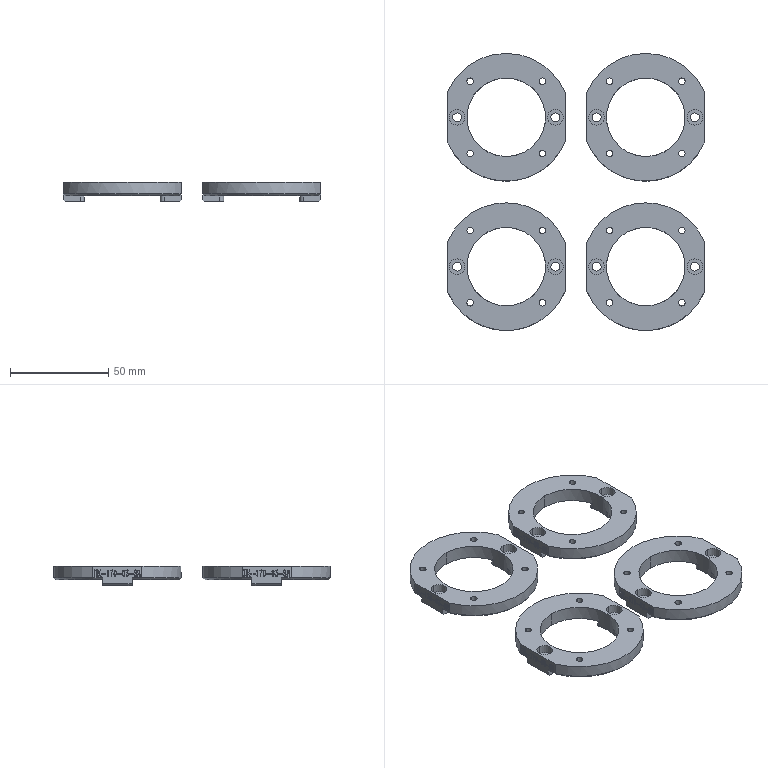NC program | NX | posted with a generic post | part box 131 x 141 x 10 mm
Lines 9684 to 11277 of 14293:
(FLOOR_WALL_COPY , TOOL : D10JING)
N19354 T14 M6
N19356 G54
N19358 G17 G0 G90 X-34.072 Y-75.973 S9500 M3
N19360 G43 Z30. H14
N19362 Z-2.
N19364 G94 G1 Z-3. F1000.
N19366 X-34.634 Y-75.
N19368 G3 X-35.5 Y-74.5 R1.
N19370 G2 X-69.103 Y-52.25 R36.5 F1500.
N19372 G1 X-69.5 Y-51.315
N19374 Y-51.
N19376 X-56.801
N19378 G3 X-49.31 Y-43.856 R7.5
N19380 X-21.69 Y-43.856 R15.
N19382 X-14.199 Y-51. R7.5
N19384 G1 X-1.5
N19386 Y-51.315
N19388 X-1.897 Y-52.25
N19390 G2 X-35.5 Y-74.5 R36.5
N19392 G1 Y-69.5
N19394 G2 X-61.351 Y-56. R31.5
N19396 G1 X-56.801
N19398 G3 X-48.703 Y-53.022 R12.5
N19400 X-22.297 Y-53.022 R20.
N19402 X-14.199 Y-56. R12.5
N19404 G1 X-9.649
N19406 G2 X-35.5 Y-69.5 R31.5
N19408 G1 Y-64.5
N19410 G2 X-50.519 Y-59.833 R26.5
N19412 G3 X-48.892 Y-59.111 R17.5
N19414 X-22.108 Y-59.111 R25.
N19416 X-20.481 Y-59.833 R17.5
N19418 G2 X-35.5 Y-64.5 R26.5
N19420 G3 X-36.366 Y-65. R1.
N19422 G1 Z-2.
N19424 G0 Z30.
N19426 X-48.796 Y-40.339
N19428 Z-2.
N19430 G1 Z-3. F1000.
N19432 X-49.643 Y-41.1
N19434 G3 X-49.953 Y-42.051 R1.
N19436 G2 X-56.801 Y-50.5 R7. F1500.
N19438 G1 X-69.5
N19440 G3 X-70.366 Y-51. R1.
N19442 G1 X-70.943 Y-52.
N19444 Z-2.
N19446 G0 Z30.
N19448 X-0.057
N19450 Z-2.
N19452 G1 Z-3. F1000.
N19454 X-0.634 Y-51.
N19456 G3 X-1.5 Y-50.5 R1.
N19458 G1 X-14.199 F1500.
N19460 G2 X-21.047 Y-42.051 R7.
N19462 G3 X-21.357 Y-41.1 R1.
N19464 G1 X-22.204 Y-40.339
N19466 Z-2.
N19468 G0 Z30.
N19470 X-36.928 Y-0.027
N19472 Z-2.
N19474 G1 Z-3. F1000.
N19476 X-36.366 Y-1.
N19478 G3 X-35.5 Y-1.5 R1.
N19480 G2 X-1.897 Y-23.75 R36.5 F1500.
N19482 G1 X-1.5 Y-24.685
N19484 Y-25.
N19486 X-14.199
N19488 G3 X-21.69 Y-32.144 R7.5
N19490 X-49.31 Y-32.144 R15.
N19492 X-56.801 Y-25. R7.5
N19494 G1 X-69.5
N19496 Y-24.685
N19498 X-69.103 Y-23.75
N19500 G2 X-35.5 Y-1.5 R36.5
N19502 G1 Y-6.5
N19504 G2 X-9.649 Y-20. R31.5
N19506 G1 X-14.199
N19508 G3 X-22.297 Y-22.978 R12.5
N19510 X-48.703 Y-22.978 R20.
N19512 X-56.801 Y-20. R12.5
N19514 G1 X-61.351
N19516 G2 X-35.5 Y-6.5 R31.5
N19518 G1 Y-11.5
N19520 G2 X-20.481 Y-16.167 R26.5
N19522 G3 X-22.108 Y-16.889 R17.5
N19524 X-48.892 Y-16.889 R25.
N19526 X-50.519 Y-16.167 R17.5
N19528 G2 X-35.5 Y-11.5 R26.5
N19530 G3 X-34.634 Y-11. R1.
N19532 G1 Z-2.
N19534 G0 Z30.
N19536 X-22.204 Y-35.661
N19538 Z-2.
N19540 G1 Z-3. F1000.
N19542 X-21.357 Y-34.9
N19544 G3 X-21.047 Y-33.949 R1.
N19546 G2 X-14.199 Y-25.5 R7. F1500.
N19548 G1 X-1.5
N19550 G3 X-0.634 Y-25. R1.
N19552 G1 X-0.057 Y-24.
N19554 Z-2.
N19556 G0 Z30.
N19558 X-70.943
N19560 Z-2.
N19562 G1 Z-3. F1000.
N19564 X-70.366 Y-25.
N19566 G3 X-69.5 Y-25.5 R1.
N19568 G1 X-56.801 F1500.
N19570 G2 X-49.953 Y-33.949 R7.
N19572 G3 X-49.643 Y-34.9 R1.
N19574 G1 X-48.796 Y-35.661
N19576 Z-2.
N19578 G0 Z30.
N19580 X36.928 Y-75.973
N19582 Z-2.
N19584 G1 Z-3. F1000.
N19586 X36.366 Y-75.
N19588 G3 X35.5 Y-74.5 R1.
N19590 G2 X1.897 Y-52.25 R36.5 F1500.
N19592 G1 X1.5 Y-51.315
N19594 Y-51.
N19596 X14.199
N19598 G3 X21.69 Y-43.856 R7.5
N19600 X49.31 Y-43.856 R15.
N19602 X56.801 Y-51. R7.5
N19604 G1 X69.5
N19606 Y-51.315
N19608 X69.103 Y-52.25
N19610 G2 X35.5 Y-74.5 R36.5
N19612 G1 Y-69.5
N19614 G2 X9.649 Y-56. R31.5
N19616 G1 X14.199
N19618 G3 X16.627 Y-55.762 R12.5
N19620 G1 X16.709
N19622 X17.324 Y-55.603
N19624 G3 X22.297 Y-53.022 R12.5
N19626 X48.703 Y-53.022 R20.
N19628 X56.801 Y-56. R12.5
N19630 G1 X61.351
N19632 G2 X35.5 Y-69.5 R31.5
N19634 G1 Y-64.5
N19636 G2 X20.481 Y-59.833 R26.5
N19638 G3 X22.108 Y-59.111 R17.5
N19640 X48.892 Y-59.111 R25.
N19642 X50.519 Y-59.833 R17.5
N19644 G2 X35.5 Y-64.5 R26.5
N19646 G3 X34.634 Y-65. R1.
N19648 G1 Z-2.
N19650 G0 Z30.
N19652 X22.204 Y-40.339
N19654 Z-2.
N19656 G1 Z-3. F1000.
N19658 X21.357 Y-41.1
N19660 G3 X21.047 Y-42.051 R1.
N19662 G2 X14.199 Y-50.5 R7. F1500.
N19664 G1 X1.5
N19666 G3 X0.634 Y-51. R1.
N19668 G1 X0.057 Y-52.
N19670 Z-2.
N19672 G0 Z30.
N19674 X70.943
N19676 Z-2.
N19678 G1 Z-3. F1000.
N19680 X70.366 Y-51.
N19682 G3 X69.5 Y-50.5 R1.
N19684 G1 X56.801 F1500.
N19686 G2 X49.953 Y-42.051 R7.
N19688 G3 X49.643 Y-41.1 R1.
N19690 G1 X48.796 Y-40.339
N19692 Z-2.
N19694 G0 Z30.
N19696 X34.072 Y-0.027
N19698 Z-2.
N19700 G1 Z-3. F1000.
N19702 X34.634 Y-1.
N19704 G3 X35.5 Y-1.5 R1.
N19706 G2 X69.103 Y-23.75 R36.5 F1500.
N19708 G1 X69.5 Y-24.685
N19710 Y-25.
N19712 X56.801
N19714 G3 X49.31 Y-32.144 R7.5
N19716 X21.69 Y-32.144 R15.
N19718 X14.199 Y-25. R7.5
N19720 G1 X1.5
N19722 Y-24.685
N19724 X1.897 Y-23.75
N19726 G2 X35.5 Y-1.5 R36.5
N19728 G1 Y-6.5
N19730 G2 X61.351 Y-20. R31.5
N19732 G1 X56.801
N19734 G3 X48.703 Y-22.978 R12.5
N19736 X22.297 Y-22.978 R20.
N19738 X14.199 Y-20. R12.5
N19740 G1 X9.649
N19742 G2 X35.5 Y-6.5 R31.5
N19744 G1 Y-11.5
N19746 G2 X50.519 Y-16.167 R26.5
N19748 G3 X48.892 Y-16.889 R17.5
N19750 X22.108 Y-16.889 R25.
N19752 X20.481 Y-16.167 R17.5
N19754 G2 X35.5 Y-11.5 R26.5
N19756 G3 X36.366 Y-11. R1.
N19758 G1 Z-2.
N19760 G0 Z30.
N19762 X48.796 Y-35.661
N19764 Z-2.
N19766 G1 Z-3. F1000.
N19768 X49.643 Y-34.9
N19770 G3 X49.953 Y-33.949 R1.
N19772 G2 X56.801 Y-25.5 R7. F1500.
N19774 G1 X69.5
N19776 G3 X70.366 Y-25. R1.
N19778 G1 X70.943 Y-24.
N19780 Z-2.
N19782 G0 Z30.
N19784 X0.057
N19786 Z-2.
N19788 G1 Z-3. F1000.
N19790 X0.634 Y-25.
N19792 G3 X1.5 Y-25.5 R1.
N19794 G1 X14.199 F1500.
N19796 G2 X21.047 Y-33.949 R7.
N19798 G3 X21.357 Y-34.9 R1.
N19800 G1 X22.204 Y-35.661
N19802 Z-2.
N19804 G0 Z30.
N19806 X36.928 Y0.027
N19808 Z-2.
N19810 G1 Z-3. F1000.
N19812 X36.366 Y1.
N19814 G3 X35.5 Y1.5 R1.
N19816 G2 X1.897 Y23.75 R36.5 F1500.
N19818 G1 X1.5 Y24.685
N19820 Y25.
N19822 X14.199
N19824 G3 X21.69 Y32.144 R7.5
N19826 X49.31 Y32.144 R15.
N19828 X56.801 Y25. R7.5
N19830 G1 X69.5
N19832 Y24.685
N19834 X69.103 Y23.75
N19836 G2 X35.5 Y1.5 R36.5
N19838 G1 Y6.5
N19840 G2 X9.649 Y20. R31.5
N19842 G1 X14.199
N19844 G3 X16.627 Y20.238 R12.5
N19846 G1 X16.709
N19848 X17.324 Y20.397
N19850 G3 X22.297 Y22.978 R12.5
N19852 X48.703 Y22.978 R20.
N19854 X56.801 Y20. R12.5
N19856 G1 X61.351
N19858 G2 X35.5 Y6.5 R31.5
N19860 G1 Y11.5
N19862 G2 X20.481 Y16.167 R26.5
N19864 G3 X22.108 Y16.889 R17.5
N19866 X48.892 Y16.889 R25.
N19868 X50.519 Y16.167 R17.5
N19870 G2 X35.5 Y11.5 R26.5
N19872 G3 X34.634 Y11. R1.
N19874 G1 Z-2.
N19876 G0 Z30.
N19878 X22.204 Y35.661
N19880 Z-2.
N19882 G1 Z-3. F1000.
N19884 X21.357 Y34.9
N19886 G3 X21.047 Y33.949 R1.
N19888 G2 X14.199 Y25.5 R7. F1500.
N19890 G1 X1.5
N19892 G3 X0.634 Y25. R1.
N19894 G1 X0.057 Y24.
N19896 Z-2.
N19898 G0 Z30.
N19900 X70.943
N19902 Z-2.
N19904 G1 Z-3. F1000.
N19906 X70.366 Y25.
N19908 G3 X69.5 Y25.5 R1.
N19910 G1 X56.801 F1500.
N19912 G2 X49.953 Y33.949 R7.
N19914 G3 X49.643 Y34.9 R1.
N19916 G1 X48.796 Y35.661
N19918 Z-2.
N19920 G0 Z30.
N19922 X34.072 Y75.973
N19924 Z-2.
N19926 G1 Z-3. F1000.
N19928 X34.634 Y75.
N19930 G3 X35.5 Y74.5 R1.
N19932 G2 X69.103 Y52.25 R36.5 F1500.
N19934 G1 X69.5 Y51.315
N19936 Y51.
N19938 X56.801
N19940 G3 X49.31 Y43.856 R7.5
N19942 X21.69 Y43.856 R15.
N19944 X14.199 Y51. R7.5
N19946 G1 X1.5
N19948 Y51.315
N19950 X1.897 Y52.25
N19952 G2 X35.5 Y74.5 R36.5
N19954 G1 Y69.5
N19956 G2 X61.351 Y56. R31.5
N19958 G1 X56.801
N19960 G3 X48.703 Y53.022 R12.5
N19962 X22.297 Y53.022 R20.
N19964 X14.199 Y56. R12.5
N19966 G1 X9.649
N19968 G2 X35.5 Y69.5 R31.5
N19970 G1 Y64.5
N19972 G2 X50.519 Y59.833 R26.5
N19974 G3 X48.892 Y59.111 R17.5
N19976 X22.108 Y59.111 R25.
N19978 X20.481 Y59.833 R17.5
N19980 G2 X35.5 Y64.5 R26.5
N19982 G3 X36.366 Y65. R1.
N19984 G1 Z-2.
N19986 G0 Z30.
N19988 X48.796 Y40.339
N19990 Z-2.
N19992 G1 Z-3. F1000.
N19994 X49.643 Y41.1
N19996 G3 X49.953 Y42.051 R1.
N19998 G2 X56.801 Y50.5 R7. F1500.
N20000 G1 X69.5
N20002 G3 X70.366 Y51. R1.
N20004 G1 X70.943 Y52.
N20006 Z-2.
N20008 G0 Z30.
N20010 X0.057
N20012 Z-2.
N20014 G1 Z-3. F1000.
N20016 X0.634 Y51.
N20018 G3 X1.5 Y50.5 R1.
N20020 G1 X14.199 F1500.
N20022 G2 X21.047 Y42.051 R7.
N20024 G3 X21.357 Y41.1 R1.
N20026 G1 X22.204 Y40.339
N20028 Z-2.
N20030 G0 Z30.
N20032 X-36.928 Y75.973
N20034 Z-2.
N20036 G1 Z-3. F1000.
N20038 X-36.366 Y75.
N20040 G3 X-35.5 Y74.5 R1.
N20042 G2 X-1.897 Y52.25 R36.5 F1500.
N20044 G1 X-1.5 Y51.315
N20046 Y51.
N20048 X-14.199
N20050 G3 X-21.69 Y43.856 R7.5
N20052 X-49.31 Y43.856 R15.
N20054 X-56.801 Y51. R7.5
N20056 G1 X-69.5
N20058 Y51.315
N20060 X-69.103 Y52.25
N20062 G2 X-35.5 Y74.5 R36.5
N20064 G1 Y69.5
N20066 G2 X-9.649 Y56. R31.5
N20068 G1 X-14.199
N20070 G3 X-22.297 Y53.022 R12.5
N20072 X-48.703 Y53.022 R20.
N20074 X-56.801 Y56. R12.5
N20076 G1 X-61.351
N20078 G2 X-35.5 Y69.5 R31.5
N20080 G1 Y64.5
N20082 G2 X-20.481 Y59.833 R26.5
N20084 G3 X-22.108 Y59.111 R17.5
N20086 X-48.892 Y59.111 R25.
N20088 X-50.519 Y59.833 R17.5
N20090 G2 X-35.5 Y64.5 R26.5
N20092 G3 X-34.634 Y65. R1.
N20094 G1 Z-2.
N20096 G0 Z30.
N20098 X-22.204 Y40.339
N20100 Z-2.
N20102 G1 Z-3. F1000.
N20104 X-21.357 Y41.1
N20106 G3 X-21.047 Y42.051 R1.
N20108 G2 X-14.199 Y50.5 R7. F1500.
N20110 G1 X-1.5
N20112 G3 X-0.634 Y51. R1.
N20114 G1 X-0.057 Y52.
N20116 Z-2.
N20118 G0 Z30.
N20120 X-70.943
N20122 Z-2.
N20124 G1 Z-3. F1000.
N20126 X-70.366 Y51.
N20128 G3 X-69.5 Y50.5 R1.
N20130 G1 X-56.801 F1500.
N20132 G2 X-49.953 Y42.051 R7.
N20134 G3 X-49.643 Y41.1 R1.
N20136 G1 X-48.796 Y40.339
N20138 Z-2.
N20140 G0 Z30.
N20142 X-34.072 Y0.027
N20144 Z-2.
N20146 G1 Z-3. F1000.
N20148 X-34.634 Y1.
N20150 G3 X-35.5 Y1.5 R1.
N20152 G2 X-69.103 Y23.75 R36.5 F1500.
N20154 G1 X-69.5 Y24.685
N20156 Y25.
N20158 X-56.801
N20160 G3 X-49.31 Y32.144 R7.5
N20162 X-21.69 Y32.144 R15.
N20164 X-14.199 Y25. R7.5
N20166 G1 X-1.5
N20168 Y24.685
N20170 X-1.897 Y23.75
N20172 G2 X-35.5 Y1.5 R36.5
N20174 G1 Y6.5
N20176 G2 X-61.351 Y20. R31.5
N20178 G1 X-56.801
N20180 G3 X-48.703 Y22.978 R12.5
N20182 X-22.297 Y22.978 R20.
N20184 X-14.199 Y20. R12.5
N20186 G1 X-9.649
N20188 G2 X-35.5 Y6.5 R31.5
N20190 G1 Y11.5
N20192 G2 X-50.519 Y16.167 R26.5
N20194 G3 X-48.892 Y16.889 R17.5
N20196 X-22.108 Y16.889 R25.
N20198 X-20.481 Y16.167 R17.5
N20200 G2 X-35.5 Y11.5 R26.5
N20202 G3 X-36.366 Y11. R1.
N20204 G1 Z-2.
N20206 G0 Z30.
N20208 X-48.796 Y35.661
N20210 Z-2.
N20212 G1 Z-3. F1000.
N20214 X-49.643 Y34.9
N20216 G3 X-49.953 Y33.949 R1.
N20218 G2 X-56.801 Y25.5 R7. F1500.
N20220 G1 X-69.5
N20222 G3 X-70.366 Y25. R1.
N20224 G1 X-70.943 Y24.
N20226 Z-2.
N20228 G0 Z30.
N20230 X-0.057
N20232 Z-2.
N20234 G1 Z-3. F1000.
N20236 X-0.634 Y25.
N20238 G3 X-1.5 Y25.5 R1.
N20240 G1 X-14.199 F1500.
N20242 G2 X-21.047 Y33.949 R7.
N20244 G3 X-21.357 Y34.9 R1.
N20246 G1 X-22.204 Y35.661
N20248 Z-2.
N20250 G0 Z30.
(HOLE_MILLING_COPY , TOOL : D10JING)
N20252 X35.5 Y38.
N20254 Z0.5
N20256 G1 X23.912 Y40.707 F1000.
N20258 G3 X20.5 Y38. R2.78
N20260 X20.5 Y38. Z-9.5 I15. J0. F1200.
N20262 X21.234 Y33.365 Z-10. R15.
N20264 X40.135 Y23.734 R15.
N20266 X21.234 Y33.365 R-15.
N20268 X25.316 Y31.845 R2.78
N20270 G1 X35.5 Y38.
N20272 G0 Z30.
N20274 X-35.5
N20276 Z0.5
N20278 G1 X-47.088 Y40.707 F1000.
N20280 G3 X-50.5 Y38. R2.78
N20282 X-50.5 Y38. Z-9.5 I15. J0. F1200.
N20284 X-49.766 Y33.365 Z-10. R15.
N20286 X-30.865 Y23.734 R15.
N20288 X-49.766 Y33.365 R-15.
N20290 X-45.684 Y31.845 R2.78
N20292 G1 X-35.5 Y38.
N20294 G0 Z30.
N20296 Y-38.
N20298 Z0.5
N20300 G1 X-47.088 Y-35.293 F1000.
N20302 G3 X-50.5 Y-38. R2.78
N20304 X-50.5 Y-38. Z-9.5 I15. J0. F1200.
N20306 X-49.766 Y-42.635 Z-10. R15.
N20308 X-30.865 Y-52.266 R15.
N20310 X-49.766 Y-42.635 R-15.
N20312 X-45.684 Y-44.155 R2.78
N20314 G1 X-35.5 Y-38.
N20316 G0 Z30.
N20318 X35.5
N20320 Z0.5
N20322 G1 X23.912 Y-35.293 F1000.
N20324 G3 X20.5 Y-38. R2.78
N20326 X20.5 Y-38. Z-9.5 I15. J0. F1200.
N20328 X21.234 Y-42.635 Z-10. R15.
N20330 X40.135 Y-52.266 R15.
N20332 X21.234 Y-42.635 R-15.
N20334 X25.316 Y-44.155 R2.78
N20336 G1 X35.5 Y-38.
N20338 G0 Z30.
N20340 M5
(DRILLING , TOOL : D6A45)
N20342 T01 M6
N20344 G54
N20346 G17 G0 G90 X-53.885 Y19.615 S5000 M3
N20348 G43 Z30. H1
N20350 G94 G81 G98 Z-4. F350. R0.
N20352 X-60.5 Y38. Z-1. R3.
N20354 X-53.885 Y56.385 Z-4. R0.
N20356 X-17.115
N20358 X-10.5 Y38. Z-1. R3.
N20360 X-17.115 Y19.615 Z-4. R0.
N20362 X17.115
N20364 X10.5 Y38. Z-1. R3.
N20366 X17.115 Y56.385 Z-4. R0.
N20368 X53.885
N20370 X60.5 Y38. Z-1. R3.
N20372 X53.885 Y19.615 Z-4. R0.
N20374 Y-19.615
N20376 X60.5 Y-38. Z-1. R3.
N20378 X53.885 Y-56.385 Z-4. R0.
N20380 X17.115
N20382 X10.5 Y-38. Z-1. R3.
N20384 X17.115 Y-19.615 Z-4. R0.
N20386 X-17.115
N20388 X-10.5 Y-38. Z-1. R3.
N20390 X-17.115 Y-56.385 Z-4. R0.
N20392 X-53.885
N20394 X-60.5 Y-38. Z-1. R3.
N20396 X-53.885 Y-19.615 Z-4. R0.
N20398 G80
N20400 G0 X-53.885 Y-19.615 Z30.
N20402 M5
(DRILLING_COPY , TOOL : 4.5ZT)
N20404 T08 M6
N20406 G54
N20408 G17 G0 G90 X60.5 Y38. S2000 M3
N20410 G43 Z30. H8
N20412 G94 G83 G98 Z-11.352 F300. Q2. R3.
N20414 X10.5
N20416 X-10.5
N20418 X-60.5
N20420 Y-38.
N20422 X-10.5
N20424 X10.5
N20426 X60.5
N20428 G80
N20430 G0 X60.5 Y-38. Z30.
N20432 M5
(DRILLING_COPY_COPY , TOOL : 3.3ZT)
N20434 T03 M6
N20436 G54
N20438 G17 G0 G90 X-53.885 Y-19.615 S2000 M3
N20440 G43 Z30. H3
N20442 G94 G83 G98 Z-12.491 F200. Q2. R0.
N20444 Y-56.385
N20446 X-17.115
N20448 X17.115
N20450 X53.885
N20452 Y-19.615
N20454 X17.115
N20456 X-17.115
N20458 Y19.615
N20460 X17.115
N20462 X53.885
N20464 Y56.385
N20466 X17.115
N20468 X-17.115
N20470 X-53.885
N20472 Y19.615
N20474 G80
N20476 G0 X-53.885 Y19.615 Z30.
N20478 M5
(PLANAR_MILL_COPY_COPY_COPY_COPY , TOOL : D6A45)
N20480 T01 M6
N20482 G54
N20484 G17 G0 G90 X-61.1 Y38.433 S9500 M3
N20486 G43 Z30. H1
N20488 Z0.
N20490 G94 G1 Z-1.5 F1250.
N20492 G3 X-61.35 Y38. R0.5
N20494 X-60.5 Y37.15 R0.85
N20496 X-61.35 Y38. R-0.85
N20498 X-61.1 Y37.567 R0.5
N20500 G1 Z0.
N20502 G0 Z30.
N20504 X-67.4 Y37.134
N20506 Z0.
N20508 G1 Z-1.5
N20510 G3 X-66.9 Y38. R1.
N20512 G1 Y45.5
N20514 G2 X-65.5 Y46.9 R1.4
N20516 G1 X-56.801
N20518 G2 X-53.509 Y42.65 R3.4
N20520 G3 X-53.509 Y33.35 R18.6
N20522 G2 X-56.801 Y29.1 R3.4
N20524 G1 X-65.5
N20526 G2 X-66.9 Y30.5 R1.4
N20528 G1 Y38.
N20530 G3 X-67.4 Y38.866 R1.
N20532 G1 Z0.
N20534 G0 Z30.
N20536 X-3.6
N20538 Z0.
N20540 G1 Z-1.5
N20542 G3 X-4.1 Y38. R1.
N20544 G1 Y30.5
N20546 G2 X-5.5 Y29.1 R1.4
N20548 G1 X-14.199
N20550 G2 X-17.491 Y33.35 R3.4
N20552 G3 X-17.491 Y42.65 R18.6
N20554 G2 X-14.199 Y46.9 R3.4
N20556 G1 X-5.5
N20558 G2 X-4.1 Y45.5 R1.4
N20560 G1 Y38.
N20562 G3 X-3.6 Y37.134 R1.
N20564 G1 Z0.
N20566 G0 Z30.
N20568 X-10.067 Y38.6
N20570 Z0.
N20572 G1 Z-1.5
N20574 G3 X-10.5 Y38.85 R0.5
N20576 X-11.35 Y38. R0.85
N20578 X-10.5 Y38.85 R-0.85
N20580 X-10.933 Y38.6 R0.5
N20582 G1 Z0.
N20584 G0 Z30.
N20586 X10.933
N20588 Z0.
N20590 G1 Z-1.5
N20592 G3 X10.5 Y38.85 R0.5
N20594 X9.65 Y38. R0.85
N20596 X10.5 Y38.85 R-0.85
N20598 X10.067 Y38.6 R0.5
N20600 G1 Z0.
N20602 G0 Z30.
N20604 X3.6 Y37.134
N20606 Z0.
N20608 G1 Z-1.5
N20610 G3 X4.1 Y38. R1.
N20612 G1 Y45.5
N20614 G2 X5.5 Y46.9 R1.4
N20616 G1 X14.199
N20618 G2 X17.491 Y42.65 R3.4
N20620 G3 X17.491 Y33.35 R18.6
N20622 G2 X14.199 Y29.1 R3.4
N20624 G1 X5.5
N20626 G2 X4.1 Y30.5 R1.4
N20628 G1 Y38.
N20630 G3 X3.6 Y38.866 R1.
N20632 G1 Z0.
N20634 G0 Z30.
N20636 X67.4
N20638 Z0.
N20640 G1 Z-1.5
N20642 G3 X66.9 Y38. R1.
N20644 G1 Y30.5
N20646 G2 X65.5 Y29.1 R1.4
N20648 G1 X56.801
N20650 G2 X53.509 Y33.35 R3.4
N20652 G3 X53.509 Y42.65 R18.6
N20654 G2 X56.801 Y46.9 R3.4
N20656 G1 X65.5
N20658 G2 X66.9 Y45.5 R1.4
N20660 G1 Y38.
N20662 G3 X67.4 Y37.134 R1.
N20664 G1 Z0.
N20666 G0 Z30.
N20668 X61.1 Y37.567
N20670 Z0.
N20672 G1 Z-1.5
N20674 G3 X61.35 Y38. R0.5
N20676 X60.5 Y38.85 R0.85
N20678 X61.35 Y38. R-0.85
N20680 X61.1 Y38.433 R0.5
N20682 G1 Z0.
N20684 G0 Z30.
N20686 Y-38.433
N20688 Z0.
N20690 G1 Z-1.5
N20692 G3 X61.35 Y-38. R0.5
N20694 X60.5 Y-37.15 R0.85
N20696 X61.35 Y-38. R-0.85
N20698 X61.1 Y-37.567 R0.5
N20700 G1 Z0.
N20702 G0 Z30.
N20704 X67.4 Y-37.134
N20706 Z0.
N20708 G1 Z-1.5
N20710 G3 X66.9 Y-38. R1.
N20712 G1 Y-45.5
N20714 G2 X65.5 Y-46.9 R1.4
N20716 G1 X56.801
N20718 G2 X53.509 Y-42.65 R3.4
N20720 G3 X53.509 Y-33.35 R18.6
N20722 G2 X56.801 Y-29.1 R3.4
N20724 G1 X65.5
N20726 G2 X66.9 Y-30.5 R1.4
N20728 G1 Y-38.
N20730 G3 X67.4 Y-38.866 R1.
N20732 G1 Z0.
N20734 G0 Z30.
N20736 X3.6
N20738 Z0.
N20740 G1 Z-1.5
N20742 G3 X4.1 Y-38. R1.
N20744 G1 Y-30.5
N20746 G2 X5.5 Y-29.1 R1.4
N20748 G1 X14.199
N20750 G2 X17.491 Y-33.35 R3.4
N20752 G3 X17.491 Y-42.65 R18.6
N20754 G2 X14.199 Y-46.9 R3.4
N20756 G1 X5.5
N20758 G2 X4.1 Y-45.5 R1.4
N20760 G1 Y-38.
N20762 G3 X3.6 Y-37.134 R1.
N20764 G1 Z0.
N20766 G0 Z30.
N20768 X10.067 Y-38.6
N20770 Z0.
N20772 G1 Z-1.5
N20774 G3 X10.5 Y-38.85 R0.5
N20776 X11.35 Y-38. R0.85
N20778 X10.5 Y-38.85 R-0.85
N20780 X10.933 Y-38.6 R0.5
N20782 G1 Z0.
N20784 G0 Z30.
N20786 X-10.933
N20788 Z0.
N20790 G1 Z-1.5
N20792 G3 X-10.5 Y-38.85 R0.5
N20794 X-9.65 Y-38. R0.85
N20796 X-10.5 Y-38.85 R-0.85
N20798 X-10.067 Y-38.6 R0.5
N20800 G1 Z0.
N20802 G0 Z30.
N20804 X-3.6 Y-37.134
N20806 Z0.
N20808 G1 Z-1.5
N20810 G3 X-4.1 Y-38. R1.
N20812 G1 Y-45.5
N20814 G2 X-5.5 Y-46.9 R1.4
N20816 G1 X-14.199
N20818 G2 X-17.491 Y-42.65 R3.4
N20820 G3 X-17.491 Y-33.35 R18.6
N20822 G2 X-14.199 Y-29.1 R3.4
N20824 G1 X-5.5
N20826 G2 X-4.1 Y-30.5 R1.4
N20828 G1 Y-38.
N20830 G3 X-3.6 Y-38.866 R1.
N20832 G1 Z0.
N20834 G0 Z30.
N20836 X-67.4
N20838 Z0.
N20840 G1 Z-1.5
N20842 G3 X-66.9 Y-38. R1.
N20844 G1 Y-30.5
N20846 G2 X-65.5 Y-29.1 R1.4
N20848 G1 X-56.801
N20850 G2 X-53.509 Y-33.35 R3.4
N20852 G3 X-53.509 Y-42.65 R18.6
N20854 G2 X-56.801 Y-46.9 R3.4
N20856 G1 X-65.5
N20858 G2 X-66.9 Y-45.5 R1.4
N20860 G1 Y-38.
N20862 G3 X-67.4 Y-37.134 R1.
N20864 G1 Z0.
N20866 G0 Z30.
N20868 X-61.1 Y-37.567
N20870 Z0.
N20872 G1 Z-1.5
N20874 G3 X-61.35 Y-38. R0.5
N20876 X-60.5 Y-38.85 R0.85
N20878 X-61.35 Y-38. R-0.85
N20880 X-61.1 Y-38.433 R0.5
N20882 G1 Z0.
N20884 G0 Z30.
(PLANAR_MILL_COPY_COPY_COPY_COPY_COPY , TOOL : D6A45)
N20886 X66.5 Y-29.634
N20888 Z0.
N20890 G1 Z-1.5
N20892 G3 X66. Y-30.5 R1.
N20894 G1 Y-45.5
N20896 G3 X66.5 Y-46.366 R1.
N20898 G1 Z0.
N20900 G0 Z30.
N20902 X4.5
N20904 Z0.
N20906 G1 Z-1.5
N20908 G3 X5. Y-45.5 R1.
N20910 G1 Y-30.5
N20912 G3 X4.5 Y-29.634 R1.
N20914 G1 Z0.
N20916 G0 Z30.
N20918 X-4.5
N20920 Z0.
N20922 G1 Z-1.5
N20924 G3 X-5. Y-30.5 R1.
N20926 G1 Y-45.5
N20928 G3 X-4.5 Y-46.366 R1.
N20930 G1 Z0.
N20932 G0 Z30.
N20934 X-66.5
N20936 Z0.
N20938 G1 Z-1.5
N20940 G3 X-66. Y-45.5 R1.
N20942 G1 Y-30.5
N20944 G3 X-66.5 Y-29.634 R1.
N20946 G1 Z0.
N20948 G0 Z30.
N20950 Y29.634
N20952 Z0.
N20954 G1 Z-1.5
N20956 G3 X-66. Y30.5 R1.
N20958 G1 Y45.5
N20960 G3 X-66.5 Y46.366 R1.
N20962 G1 Z0.
N20964 G0 Z30.
N20966 X-4.5
N20968 Z0.
N20970 G1 Z-1.5
N20972 G3 X-5. Y45.5 R1.
N20974 G1 Y30.5
N20976 G3 X-4.5 Y29.634 R1.
N20978 G1 Z0.
N20980 G0 Z30.
N20982 X4.5
N20984 Z0.
N20986 G1 Z-1.5
N20988 G3 X5. Y30.5 R1.
N20990 G1 Y45.5
N20992 G3 X4.5 Y46.366 R1.
N20994 G1 Z0.
N20996 G0 Z30.
N20998 X66.5
N21000 Z0.
N21002 G1 Z-1.5
N21004 G3 X66. Y45.5 R1.
N21006 G1 Y30.5
N21008 G3 X66.5 Y29.634 R1.
N21010 G1 Z0.
N21012 G0 Z30.
(PLANAR_MILL_COPY_COPY_COPY_COPY_COPY_COPY , TOOL : D6A45)
N21014 X53.843 Y-56.635
N21016 Z-3.
N21018 G1 X54.011 Z-3.045
N21020 X54.135 Y-56.511 Z-3.092
N21022 Y-56.259 Z-3.159
N21024 X54.011 Y-56.135 Z-3.206
N21026 X53.759 Z-3.274
N21028 X53.635 Y-56.259 Z-3.321
N21030 Y-56.511 Z-3.389
N21032 X53.759 Y-56.635 Z-3.435
N21034 X54.011 Z-3.503
N21036 X54.135 Y-56.511 Z-3.55
N21038 Y-56.259 Z-3.618
N21040 X54.011 Y-56.135 Z-3.665
N21042 X53.759 Z-3.732
N21044 X53.635 Y-56.259 Z-3.779
N21046 Y-56.511 Z-3.847
N21048 X53.759 Y-56.635 Z-3.894
N21050 X54.011 Z-3.961
N21052 X54.135 Y-56.511 Z-4.008
N21054 Y-56.259 Z-4.076
N21056 X54.011 Y-56.135 Z-4.123
N21058 X53.759 Z-4.19
N21060 X53.635 Y-56.259 Z-4.237
N21062 Y-56.511 Z-4.305
N21064 X53.759 Y-56.635 Z-4.352
N21066 X54.011 Z-4.419
N21068 X54.135 Y-56.511 Z-4.466
N21070 Y-56.385 Z-4.5
N21072 G3 X53.885 Y-56.135 R0.25
N21074 X54.135 Y-56.385 R-0.25
N21076 X53.885 Y-56.318 R0.5
N21078 G1 Z-3.
N21080 G0 Z30.
N21082 X16.865 Y-56.343
N21084 Z-3.
N21086 G1 Y-56.511 Z-3.045
N21088 X16.989 Y-56.635 Z-3.092
N21090 X17.241 Z-3.159
N21092 X17.365 Y-56.511 Z-3.206
N21094 Y-56.259 Z-3.274
N21096 X17.241 Y-56.135 Z-3.321
N21098 X16.989 Z-3.389
N21100 X16.865 Y-56.259 Z-3.435
N21102 Y-56.511 Z-3.503
N21104 X16.989 Y-56.635 Z-3.55
N21106 X17.241 Z-3.618
N21108 X17.365 Y-56.511 Z-3.665
N21110 Y-56.259 Z-3.732
N21112 X17.241 Y-56.135 Z-3.779
N21114 X16.989 Z-3.847
N21116 X16.865 Y-56.259 Z-3.894
N21118 Y-56.511 Z-3.961
N21120 X16.989 Y-56.635 Z-4.008
N21122 X17.241 Z-4.076
N21124 X17.365 Y-56.511 Z-4.123
N21126 Y-56.259 Z-4.19
N21128 X17.241 Y-56.135 Z-4.237
N21130 X16.989 Z-4.305
N21132 X16.865 Y-56.259 Z-4.352
N21134 Y-56.511 Z-4.419
N21136 X16.989 Y-56.635 Z-4.466
N21138 X17.115 Z-4.5
N21140 G3 X17.365 Y-56.385 R0.25
N21142 X17.115 Y-56.635 R-0.25
N21144 X17.182 Y-56.385 R0.5
N21146 G1 Z-3.
N21148 G0 Z30.
N21150 X-17.365 Y-56.343
N21152 Z-3.
N21154 G1 Y-56.511 Z-3.045
N21156 X-17.241 Y-56.635 Z-3.092
N21158 X-16.989 Z-3.159
N21160 X-16.865 Y-56.511 Z-3.206
N21162 Y-56.259 Z-3.274
N21164 X-16.989 Y-56.135 Z-3.321
N21166 X-17.241 Z-3.389
N21168 X-17.365 Y-56.259 Z-3.435
N21170 Y-56.511 Z-3.503
N21172 X-17.241 Y-56.635 Z-3.55
N21174 X-16.989 Z-3.618
N21176 X-16.865 Y-56.511 Z-3.665
N21178 Y-56.259 Z-3.732
N21180 X-16.989 Y-56.135 Z-3.779
N21182 X-17.241 Z-3.847
N21184 X-17.365 Y-56.259 Z-3.894
N21186 Y-56.511 Z-3.961
N21188 X-17.241 Y-56.635 Z-4.008
N21190 X-16.989 Z-4.076
N21192 X-16.865 Y-56.511 Z-4.123
N21194 Y-56.259 Z-4.19
N21196 X-16.989 Y-56.135 Z-4.237
N21198 X-17.241 Z-4.305
N21200 X-17.365 Y-56.259 Z-4.352
N21202 Y-56.511 Z-4.419
N21204 X-17.241 Y-56.635 Z-4.466
N21206 X-17.115 Z-4.5
N21208 G3 X-16.865 Y-56.385 R0.25
N21210 X-17.115 Y-56.635 R-0.25
N21212 X-17.048 Y-56.385 R0.5
N21214 G1 Z-3.
N21216 G0 Z30.
N21218 X-53.843 Y-56.135
N21220 Z-3.
N21222 G1 X-54.011 Z-3.045
N21224 X-54.135 Y-56.259 Z-3.092
N21226 Y-56.511 Z-3.159
N21228 X-54.011 Y-56.635 Z-3.206
N21230 X-53.759 Z-3.274
N21232 X-53.635 Y-56.511 Z-3.321
N21234 Y-56.259 Z-3.389
N21236 X-53.759 Y-56.135 Z-3.435
N21238 X-54.011 Z-3.503
N21240 X-54.135 Y-56.259 Z-3.55
N21242 Y-56.511 Z-3.618
N21244 X-54.011 Y-56.635 Z-3.665
N21246 X-53.759 Z-3.732
N21248 X-53.635 Y-56.511 Z-3.779
N21250 Y-56.259 Z-3.847
N21252 X-53.759 Y-56.135 Z-3.894
N21254 X-54.011 Z-3.961
N21256 X-54.135 Y-56.259 Z-4.008
N21258 Y-56.511 Z-4.076
N21260 X-54.011 Y-56.635 Z-4.123
N21262 X-53.759 Z-4.19
N21264 X-53.635 Y-56.511 Z-4.237
N21266 Y-56.259 Z-4.305
N21268 X-53.759 Y-56.135 Z-4.352
N21270 X-54.011 Z-4.419
N21272 X-54.135 Y-56.259 Z-4.466
N21274 Y-56.385 Z-4.5
N21276 G3 X-53.885 Y-56.635 R0.25
N21278 X-54.135 Y-56.385 R-0.25
N21280 X-53.885 Y-56.452 R0.5
N21282 G1 Z-3.
N21284 G0 Z30.
N21286 X-53.843 Y-19.365
N21288 Z-3.
N21290 G1 X-54.011 Z-3.045
N21292 X-54.135 Y-19.489 Z-3.092
N21294 Y-19.741 Z-3.159
N21296 X-54.011 Y-19.865 Z-3.206
N21298 X-53.759 Z-3.274
N21300 X-53.635 Y-19.741 Z-3.321
N21302 Y-19.489 Z-3.389
N21304 X-53.759 Y-19.365 Z-3.435
N21306 X-54.011 Z-3.503
N21308 X-54.135 Y-19.489 Z-3.55
N21310 Y-19.741 Z-3.618
N21312 X-54.011 Y-19.865 Z-3.665
N21314 X-53.759 Z-3.732
N21316 X-53.635 Y-19.741 Z-3.779
N21318 Y-19.489 Z-3.847
N21320 X-53.759 Y-19.365 Z-3.894
N21322 X-54.011 Z-3.961
N21324 X-54.135 Y-19.489 Z-4.008
N21326 Y-19.741 Z-4.076
N21328 X-54.011 Y-19.865 Z-4.123
N21330 X-53.759 Z-4.19
N21332 X-53.635 Y-19.741 Z-4.237
N21334 Y-19.489 Z-4.305
N21336 X-53.759 Y-19.365 Z-4.352
N21338 X-54.011 Z-4.419
N21340 X-54.135 Y-19.489 Z-4.466
N21342 Y-19.615 Z-4.5
N21344 G3 X-53.885 Y-19.865 R0.25
N21346 X-54.135 Y-19.615 R-0.25
N21348 X-53.885 Y-19.682 R0.5
N21350 G1 Z-3.
N21352 G0 Z30.
N21354 X-50.55 Y-45.91
N21356 Z-3.
N21358 G1 Z-4.5
N21360 X-51.231 Y-45.893
N21362 G3 X-52.11 Y-46.371 R1.
N21364 X-18.89 Y-46.371 R18.6
N21366 X-19.769 Y-45.893 R1.
N21368 G1 X-20.45 Y-45.91
N21370 Z-3.
N21372 G0 Z30.
N21374 Y-30.09
N21376 Z-3.
N21378 G1 Z-4.5
N21380 X-19.769 Y-30.107
N21382 G3 X-18.89 Y-29.629 R1.
N21384 X-52.11 Y-29.629 R18.6
N21386 X-51.231 Y-30.107 R1.
N21388 G1 X-50.55 Y-30.09
N21390 Z-3.
N21392 G0 Z30.
N21394 X-17.074 Y-19.365
N21396 Z-3.
N21398 G1 X-17.241 Z-3.045
N21400 X-17.365 Y-19.489 Z-3.092
N21402 Y-19.741 Z-3.159
N21404 X-17.241 Y-19.865 Z-3.206
N21406 X-16.989 Z-3.274
N21408 X-16.865 Y-19.741 Z-3.321
N21410 Y-19.489 Z-3.389
N21412 X-16.989 Y-19.365 Z-3.435
N21414 X-17.241 Z-3.503
N21416 X-17.365 Y-19.489 Z-3.55
N21418 Y-19.741 Z-3.618
N21420 X-17.241 Y-19.865 Z-3.665
N21422 X-16.989 Z-3.732
N21424 X-16.865 Y-19.741 Z-3.779
N21426 Y-19.489 Z-3.847
N21428 X-16.989 Y-19.365 Z-3.894
N21430 X-17.241 Z-3.961
N21432 X-17.365 Y-19.489 Z-4.008
N21434 Y-19.741 Z-4.076
N21436 X-17.241 Y-19.865 Z-4.123
N21438 X-16.989 Z-4.19
N21440 X-16.865 Y-19.741 Z-4.237
N21442 Y-19.489 Z-4.305
N21444 X-16.989 Y-19.365 Z-4.352
N21446 X-17.241 Z-4.419
N21448 X-17.365 Y-19.489 Z-4.466
N21450 Y-19.615 Z-4.5
N21452 G3 X-17.115 Y-19.865 R0.25
N21454 X-17.365 Y-19.615 R-0.25
N21456 X-17.115 Y-19.682 R0.5
N21458 G1 Z-3.
N21460 G0 Z30.
N21462 X17.074 Y-19.865
N21464 Z-3.
N21466 G1 X17.241 Z-3.045
N21468 X17.365 Y-19.741 Z-3.092
N21470 Y-19.489 Z-3.159
N21472 X17.241 Y-19.365 Z-3.206
N21474 X16.989 Z-3.274
N21476 X16.865 Y-19.489 Z-3.321
N21478 Y-19.741 Z-3.389
N21480 X16.989 Y-19.865 Z-3.435
N21482 X17.241 Z-3.503
N21484 X17.365 Y-19.741 Z-3.55
N21486 Y-19.489 Z-3.618
N21488 X17.241 Y-19.365 Z-3.665
N21490 X16.989 Z-3.732
N21492 X16.865 Y-19.489 Z-3.779
N21494 Y-19.741 Z-3.847
N21496 X16.989 Y-19.865 Z-3.894
N21498 X17.241 Z-3.961
N21500 X17.365 Y-19.741 Z-4.008
N21502 Y-19.489 Z-4.076
N21504 X17.241 Y-19.365 Z-4.123
N21506 X16.989 Z-4.19
N21508 X16.865 Y-19.489 Z-4.237
N21510 Y-19.741 Z-4.305
N21512 X16.989 Y-19.865 Z-4.352
N21514 X17.241 Z-4.419
N21516 X17.365 Y-19.741 Z-4.466
N21518 Y-19.615 Z-4.5
N21520 G3 X17.115 Y-19.365 R0.25
N21522 X17.365 Y-19.615 R-0.25
N21524 X17.115 Y-19.548 R0.5
N21526 G1 Z-3.
N21528 G0 Z30.
N21530 X20.45 Y-45.91
N21532 Z-3.
N21534 G1 Z-4.5
N21536 X19.769 Y-45.893
N21538 G3 X18.89 Y-46.371 R1.
N21540 X52.11 Y-46.371 R18.6
N21542 X51.231 Y-45.893 R1.
N21544 G1 X50.55 Y-45.91
N21546 Z-3.
N21548 G0 Z30.
N21550 Y-30.09
N21552 Z-3.
N21554 G1 Z-4.5
N21556 X51.231 Y-30.107
N21558 G3 X52.11 Y-29.629 R1.
N21560 X18.89 Y-29.629 R18.6
N21562 X19.769 Y-30.107 R1.
N21564 G1 X20.45 Y-30.09
N21566 Z-3.
N21568 G0 Z30.
N21570 X53.843 Y-19.865
N21572 Z-3.
N21574 G1 X54.011 Z-3.045
N21576 X54.135 Y-19.741 Z-3.092
N21578 Y-19.489 Z-3.159
N21580 X54.011 Y-19.365 Z-3.206
N21582 X53.759 Z-3.274
N21584 X53.635 Y-19.489 Z-3.321
N21586 Y-19.741 Z-3.389
N21588 X53.759 Y-19.865 Z-3.435
N21590 X54.011 Z-3.503
N21592 X54.135 Y-19.741 Z-3.55
N21594 Y-19.489 Z-3.618
N21596 X54.011 Y-19.365 Z-3.665
N21598 X53.759 Z-3.732
N21600 X53.635 Y-19.489 Z-3.779
N21602 Y-19.741 Z-3.847
N21604 X53.759 Y-19.865 Z-3.894
N21606 X54.011 Z-3.961
N21608 X54.135 Y-19.741 Z-4.008
N21610 Y-19.489 Z-4.076
N21612 X54.011 Y-19.365 Z-4.123
N21614 X53.759 Z-4.19
N21616 X53.635 Y-19.489 Z-4.237
N21618 Y-19.741 Z-4.305
N21620 X53.759 Y-19.865 Z-4.352
N21622 X54.011 Z-4.419
N21624 X54.135 Y-19.741 Z-4.466
N21626 Y-19.615 Z-4.5
N21628 G3 X53.885 Y-19.365 R0.25
N21630 X54.135 Y-19.615 R-0.25
N21632 X53.885 Y-19.548 R0.5
N21634 G1 Z-3.
N21636 G0 Z30.
N21638 X53.843 Y19.365
N21640 Z-3.
N21642 G1 X54.011 Z-3.045
N21644 X54.135 Y19.489 Z-3.092
N21646 Y19.741 Z-3.159
N21648 X54.011 Y19.865 Z-3.206
N21650 X53.759 Z-3.274
N21652 X53.635 Y19.741 Z-3.321
N21654 Y19.489 Z-3.389
N21656 X53.759 Y19.365 Z-3.435
N21658 X54.011 Z-3.503
N21660 X54.135 Y19.489 Z-3.55
N21662 Y19.741 Z-3.618
N21664 X54.011 Y19.865 Z-3.665
N21666 X53.759 Z-3.732
N21668 X53.635 Y19.741 Z-3.779
N21670 Y19.489 Z-3.847
N21672 X53.759 Y19.365 Z-3.894
N21674 X54.011 Z-3.961
N21676 X54.135 Y19.489 Z-4.008
N21678 Y19.741 Z-4.076
N21680 X54.011 Y19.865 Z-4.123
N21682 X53.759 Z-4.19
N21684 X53.635 Y19.741 Z-4.237
N21686 Y19.489 Z-4.305
N21688 X53.759 Y19.365 Z-4.352
N21690 X54.011 Z-4.419
N21692 X54.135 Y19.489 Z-4.466
N21694 Y19.615 Z-4.5
N21696 G3 X53.885 Y19.865 R0.25
N21698 X54.135 Y19.615 R-0.25
N21700 X53.885 Y19.682 R0.5
N21702 G1 Z-3.
N21704 G0 Z30.
N21706 X53.843 Y56.135
N21708 Z-3.
N21710 G1 X54.011 Z-3.045
N21712 X54.135 Y56.259 Z-3.092
N21714 Y56.511 Z-3.159
N21716 X54.011 Y56.635 Z-3.206
N21718 X53.759 Z-3.274
N21720 X53.635 Y56.511 Z-3.321
N21722 Y56.259 Z-3.389
N21724 X53.759 Y56.135 Z-3.435
N21726 X54.011 Z-3.503
N21728 X54.135 Y56.259 Z-3.55
N21730 Y56.511 Z-3.618
N21732 X54.011 Y56.635 Z-3.665
N21734 X53.759 Z-3.732
N21736 X53.635 Y56.511 Z-3.779
N21738 Y56.259 Z-3.847
N21740 X53.759 Y56.135 Z-3.894
N21742 X54.011 Z-3.961
N21744 X54.135 Y56.259 Z-4.008
N21746 Y56.511 Z-4.076
N21748 X54.011 Y56.635 Z-4.123
N21750 X53.759 Z-4.19
N21752 X53.635 Y56.511 Z-4.237
N21754 Y56.259 Z-4.305
N21756 X53.759 Y56.135 Z-4.352
N21758 X54.011 Z-4.419
N21760 X54.135 Y56.259 Z-4.466
N21762 Y56.385 Z-4.5
N21764 G3 X53.885 Y56.635 R0.25
N21766 X54.135 Y56.385 R-0.25
N21768 X53.885 Y56.452 R0.5
N21770 G1 Z-3.
N21772 G0 Z30.
N21774 X50.55 Y45.91
N21776 Z-3.
N21778 G1 Z-4.5
N21780 X51.231 Y45.893
N21782 G3 X52.11 Y46.371 R1.
N21784 X18.89 Y46.371 R18.6
N21786 X19.769 Y45.893 R1.
N21788 G1 X20.45 Y45.91
N21790 Z-3.
N21792 G0 Z30.
N21794 Y30.09
N21796 Z-3.
N21798 G1 Z-4.5
N21800 X19.769 Y30.107
N21802 G3 X18.89 Y29.629 R1.
N21804 X52.11 Y29.629 R18.6
N21806 X51.231 Y30.107 R1.
N21808 G1 X50.55 Y30.09
N21810 Z-3.
N21812 G0 Z30.
N21814 X17.365 Y56.343
N21816 Z-3.
N21818 G1 Y56.511 Z-3.045
N21820 X17.241 Y56.635 Z-3.092
N21822 X16.989 Z-3.159
N21824 X16.865 Y56.511 Z-3.206
N21826 Y56.259 Z-3.274
N21828 X16.989 Y56.135 Z-3.321
N21830 X17.241 Z-3.389
N21832 X17.365 Y56.259 Z-3.435
N21834 Y56.511 Z-3.503
N21836 X17.241 Y56.635 Z-3.55
N21838 X16.989 Z-3.618
N21840 X16.865 Y56.511 Z-3.665
N21842 Y56.259 Z-3.732
N21844 X16.989 Y56.135 Z-3.779
N21846 X17.241 Z-3.847
N21848 X17.365 Y56.259 Z-3.894
N21850 Y56.511 Z-3.961
N21852 X17.241 Y56.635 Z-4.008
N21854 X16.989 Z-4.076
N21856 X16.865 Y56.511 Z-4.123
N21858 Y56.259 Z-4.19
N21860 X16.989 Y56.135 Z-4.237
N21862 X17.241 Z-4.305
N21864 X17.365 Y56.259 Z-4.352
N21866 Y56.511 Z-4.419
N21868 X17.241 Y56.635 Z-4.466
N21870 X17.115 Z-4.5
N21872 G3 X16.865 Y56.385 R0.25
N21874 X17.115 Y56.635 R-0.25
N21876 X17.048 Y56.385 R0.5
N21878 G1 Z-3.
N21880 G0 Z30.
N21882 X-16.865 Y56.343
N21884 Z-3.
N21886 G1 Y56.511 Z-3.045
N21888 X-16.989 Y56.635 Z-3.092
N21890 X-17.241 Z-3.159
N21892 X-17.365 Y56.511 Z-3.206
N21894 Y56.259 Z-3.274
N21896 X-17.241 Y56.135 Z-3.321
N21898 X-16.989 Z-3.389
N21900 X-16.865 Y56.259 Z-3.435
N21902 Y56.511 Z-3.503
N21904 X-16.989 Y56.635 Z-3.55
N21906 X-17.241 Z-3.618
N21908 X-17.365 Y56.511 Z-3.665
N21910 Y56.259 Z-3.732
N21912 X-17.241 Y56.135 Z-3.779
N21914 X-16.989 Z-3.847
N21916 X-16.865 Y56.259 Z-3.894
N21918 Y56.511 Z-3.961
N21920 X-16.989 Y56.635 Z-4.008
N21922 X-17.241 Z-4.076
N21924 X-17.365 Y56.511 Z-4.123
N21926 Y56.259 Z-4.19
N21928 X-17.241 Y56.135 Z-4.237
N21930 X-16.989 Z-4.305
N21932 X-16.865 Y56.259 Z-4.352
N21934 Y56.511 Z-4.419
N21936 X-16.989 Y56.635 Z-4.466
N21938 X-17.115 Z-4.5
N21940 G3 X-17.365 Y56.385 R0.25
N21942 X-17.115 Y56.635 R-0.25
N21944 X-17.182 Y56.385 R0.5
N21946 G1 Z-3.
N21948 G0 Z30.
N21950 X-53.843 Y56.635
N21952 Z-3.
N21954 G1 X-54.011 Z-3.045
N21956 X-54.135 Y56.511 Z-3.092
N21958 Y56.259 Z-3.159
N21960 X-54.011 Y56.135 Z-3.206
N21962 X-53.759 Z-3.274
N21964 X-53.635 Y56.259 Z-3.321
N21966 Y56.511 Z-3.389
N21968 X-53.759 Y56.635 Z-3.435
N21970 X-54.011 Z-3.503
N21972 X-54.135 Y56.511 Z-3.55
N21974 Y56.259 Z-3.618
N21976 X-54.011 Y56.135 Z-3.665
N21978 X-53.759 Z-3.732
N21980 X-53.635 Y56.259 Z-3.779
N21982 Y56.511 Z-3.847
N21984 X-53.759 Y56.635 Z-3.894
N21986 X-54.011 Z-3.961
N21988 X-54.135 Y56.511 Z-4.008
N21990 Y56.259 Z-4.076
N21992 X-54.011 Y56.135 Z-4.123
N21994 X-53.759 Z-4.19
N21996 X-53.635 Y56.259 Z-4.237
N21998 Y56.511 Z-4.305
N22000 X-53.759 Y56.635 Z-4.352
N22002 X-54.011 Z-4.419
N22004 X-54.135 Y56.511 Z-4.466
N22006 Y56.385 Z-4.5
N22008 G3 X-53.885 Y56.135 R0.25
N22010 X-54.135 Y56.385 R-0.25
N22012 X-53.885 Y56.318 R0.5
N22014 G1 Z-3.
N22016 G0 Z30.
N22018 X-50.55 Y30.09
N22020 Z-3.
N22022 G1 Z-4.5
N22024 X-51.231 Y30.107
N22026 G3 X-52.11 Y29.629 R1.
N22028 X-18.89 Y29.629 R18.6
N22030 X-19.769 Y30.107 R1.
N22032 G1 X-20.45 Y30.09
N22034 Z-3.
N22036 G0 Z30.
N22038 Y45.91
N22040 Z-3.
N22042 G1 Z-4.5
N22044 X-19.769 Y45.893
N22046 G3 X-18.89 Y46.371 R1.
N22048 X-52.11 Y46.371 R18.6
N22050 X-51.231 Y45.893 R1.
N22052 G1 X-50.55 Y45.91
N22054 Z-3.
N22056 G0 Z30.
N22058 X-53.843 Y19.865
N22060 Z-3.
N22062 G1 X-54.011 Z-3.045
N22064 X-54.135 Y19.741 Z-3.092
N22066 Y19.489 Z-3.159
N22068 X-54.011 Y19.365 Z-3.206
N22070 X-53.759 Z-3.274
N22072 X-53.635 Y19.489 Z-3.321
N22074 Y19.741 Z-3.389
N22076 X-53.759 Y19.865 Z-3.435
N22078 X-54.011 Z-3.503
N22080 X-54.135 Y19.741 Z-3.55
N22082 Y19.489 Z-3.618
N22084 X-54.011 Y19.365 Z-3.665
N22086 X-53.759 Z-3.732
N22088 X-53.635 Y19.489 Z-3.779
N22090 Y19.741 Z-3.847
N22092 X-53.759 Y19.865 Z-3.894
N22094 X-54.011 Z-3.961
N22096 X-54.135 Y19.741 Z-4.008
N22098 Y19.489 Z-4.076
N22100 X-54.011 Y19.365 Z-4.123
N22102 X-53.759 Z-4.19
N22104 X-53.635 Y19.489 Z-4.237
N22106 Y19.741 Z-4.305
N22108 X-53.759 Y19.865 Z-4.352
N22110 X-54.011 Z-4.419
N22112 X-54.135 Y19.741 Z-4.466
N22114 Y19.615 Z-4.5
N22116 G3 X-53.885 Y19.365 R0.25
N22118 X-54.135 Y19.615 R-0.25
N22120 X-53.885 Y19.548 R0.5
N22122 G1 Z-3.
N22124 G0 Z30.
N22126 X-17.074 Y19.865
N22128 Z-3.
N22130 G1 X-17.241 Z-3.045
N22132 X-17.365 Y19.741 Z-3.092
N22134 Y19.489 Z-3.159
N22136 X-17.241 Y19.365 Z-3.206
N22138 X-16.989 Z-3.274
N22140 X-16.865 Y19.489 Z-3.321
N22142 Y19.741 Z-3.389
N22144 X-16.989 Y19.865 Z-3.435
N22146 X-17.241 Z-3.503
N22148 X-17.365 Y19.741 Z-3.55
N22150 Y19.489 Z-3.618
N22152 X-17.241 Y19.365 Z-3.665
N22154 X-16.989 Z-3.732
N22156 X-16.865 Y19.489 Z-3.779
N22158 Y19.741 Z-3.847
N22160 X-16.989 Y19.865 Z-3.894
N22162 X-17.241 Z-3.961
N22164 X-17.365 Y19.741 Z-4.008
N22166 Y19.489 Z-4.076
N22168 X-17.241 Y19.365 Z-4.123
N22170 X-16.989 Z-4.19
N22172 X-16.865 Y19.489 Z-4.237
N22174 Y19.741 Z-4.305
N22176 X-16.989 Y19.865 Z-4.352
N22178 X-17.241 Z-4.419
N22180 X-17.365 Y19.741 Z-4.466
N22182 Y19.615 Z-4.5
N22184 G3 X-17.115 Y19.365 R0.25
N22186 X-17.365 Y19.615 R-0.25
N22188 X-17.115 Y19.548 R0.5
N22190 G1 Z-3.
N22192 G0 Z30.
N22194 X17.074 Y19.365
N22196 Z-3.
N22198 G1 X17.241 Z-3.045
N22200 X17.365 Y19.489 Z-3.092
N22202 Y19.741 Z-3.159
N22204 X17.241 Y19.865 Z-3.206
N22206 X16.989 Z-3.274
N22208 X16.865 Y19.741 Z-3.321
N22210 Y19.489 Z-3.389
N22212 X16.989 Y19.365 Z-3.435
N22214 X17.241 Z-3.503
N22216 X17.365 Y19.489 Z-3.55
N22218 Y19.741 Z-3.618
N22220 X17.241 Y19.865 Z-3.665
N22222 X16.989 Z-3.732
N22224 X16.865 Y19.741 Z-3.779
N22226 Y19.489 Z-3.847
N22228 X16.989 Y19.365 Z-3.894
N22230 X17.241 Z-3.961
N22232 X17.365 Y19.489 Z-4.008
N22234 Y19.741 Z-4.076
N22236 X17.241 Y19.865 Z-4.123
N22238 X16.989 Z-4.19
N22240 X16.865 Y19.741 Z-4.237
N22242 Y19.489 Z-4.305
N22244 X16.989 Y19.365 Z-4.352
N22246 X17.241 Z-4.419
N22248 X17.365 Y19.489 Z-4.466
N22250 Y19.615 Z-4.5
N22252 G3 X17.115 Y19.865 R0.25
N22254 X17.365 Y19.615 R-0.25
N22256 X17.115 Y19.682 R0.5
N22258 G1 Z-3.
N22260 G0 Z30.
(PLANAR_MILL_COPY_COPY_COPY_COPY_COPY_COPY_COPY , TOOL : D6A45)
N22262 X3.679 Y49.833
N22264 Z-3.
N22266 G1 Z-4.5
N22268 X4.071 Y49.335
N22270 G3 X5. Y48.964 R1.
N22272 G1 Y50.298
N22274 G2 X5.119 Y50.884 R1.5
N22276 X65.881 Y50.884 R33.
N22278 X66. Y50.298 R1.5
N22280 G1 Y48.964
N22282 G3 X66.929 Y49.335 R1.
N22284 G1 X67.321 Y49.833
N22286 Z-3.
N22288 G0 Z30.
N22290 Y26.167
N22292 Z-3.
N22294 G1 Z-4.5
N22296 X66.929 Y26.665
N22298 G3 X66. Y27.036 R1.
N22300 G1 Y25.702
N22302 G2 X65.881 Y25.116 R1.5
N22304 X5.119 Y25.116 R33.
N22306 X5. Y25.702 R1.5
N22308 G1 Y27.036
N22310 G3 X4.071 Y26.665 R1.
N22312 G1 X3.679 Y26.167
N22314 Z-3.
N22316 G0 Z30.
N22318 X-3.679
N22320 Z-3.
N22322 G1 Z-4.5
N22324 X-4.071 Y26.665
N22326 G3 X-5. Y27.036 R1.
N22328 G1 Y25.702
N22330 G2 X-5.119 Y25.116 R1.5
N22332 X-65.881 Y25.116 R33.
N22334 X-66. Y25.702 R1.5
N22336 G1 Y27.036
N22338 G3 X-66.929 Y26.665 R1.
N22340 G1 X-67.321 Y26.167
N22342 Z-3.
N22344 G0 Z30.
N22346 Y49.833
N22348 Z-3.
N22350 G1 Z-4.5
N22352 X-66.929 Y49.335
N22354 G3 X-66. Y48.964 R1.
N22356 G1 Y50.298
N22358 G2 X-65.881 Y50.884 R1.5
N22360 X-5.119 Y50.884 R33.
N22362 X-5. Y50.298 R1.5
N22364 G1 Y48.964
N22366 G3 X-4.071 Y49.335 R1.
N22368 G1 X-3.679 Y49.833
N22370 Z-3.
N22372 G0 Z30.
N22374 X3.679 Y-26.167
N22376 Z-3.
N22378 G1 Z-4.5
N22380 X4.071 Y-26.665
N22382 G3 X5. Y-27.036 R1.
N22384 G1 Y-25.702
N22386 G2 X5.119 Y-25.116 R1.5
N22388 X65.881 Y-25.116 R33.
N22390 X66. Y-25.702 R1.5
N22392 G1 Y-27.036
N22394 G3 X66.929 Y-26.665 R1.
N22396 G1 X67.321 Y-26.167
N22398 Z-3.
N22400 G0 Z30.
N22402 Y-49.833
N22404 Z-3.
N22406 G1 Z-4.5
N22408 X66.929 Y-49.335
N22410 G3 X66. Y-48.964 R1.
N22412 G1 Y-50.298
N22414 G2 X65.881 Y-50.884 R1.5
N22416 X5.119 Y-50.884 R33.
N22418 X5. Y-50.298 R1.5
N22420 G1 Y-48.964
N22422 G3 X4.071 Y-49.335 R1.
N22424 G1 X3.679 Y-49.833
N22426 Z-3.
N22428 G0 Z30.
N22430 X-3.679
N22432 Z-3.
N22434 G1 Z-4.5
N22436 X-4.071 Y-49.335
N22438 G3 X-5. Y-48.964 R1.
N22440 G1 Y-50.298
N22442 G2 X-5.119 Y-50.884 R1.5
N22444 X-65.881 Y-50.884 R33.
N22446 X-66. Y-50.298 R1.5
N22448 G1 Y-48.964
N22450 G3 X-66.929 Y-49.335 R1.
N22452 G1 X-67.321 Y-49.833
N22454 Z-3.
N22456 G0 Z30.
N22458 Y-26.167
N22460 Z-3.
N22462 G1 Z-4.5
N22464 X-66.929 Y-26.665
N22466 G3 X-66. Y-27.036 R1.
N22468 G1 Y-25.702
N22470 G2 X-65.881 Y-25.116 R1.5
N22472 X-5.119 Y-25.116 R33.
N22474 X-5. Y-25.702 R1.5
N22476 G1 Y-27.036
N22478 G3 X-4.071 Y-26.665 R1.
N22480 G1 X-3.679 Y-26.167
N22482 Z-3.
N22484 G0 Z30.
N22486 M5